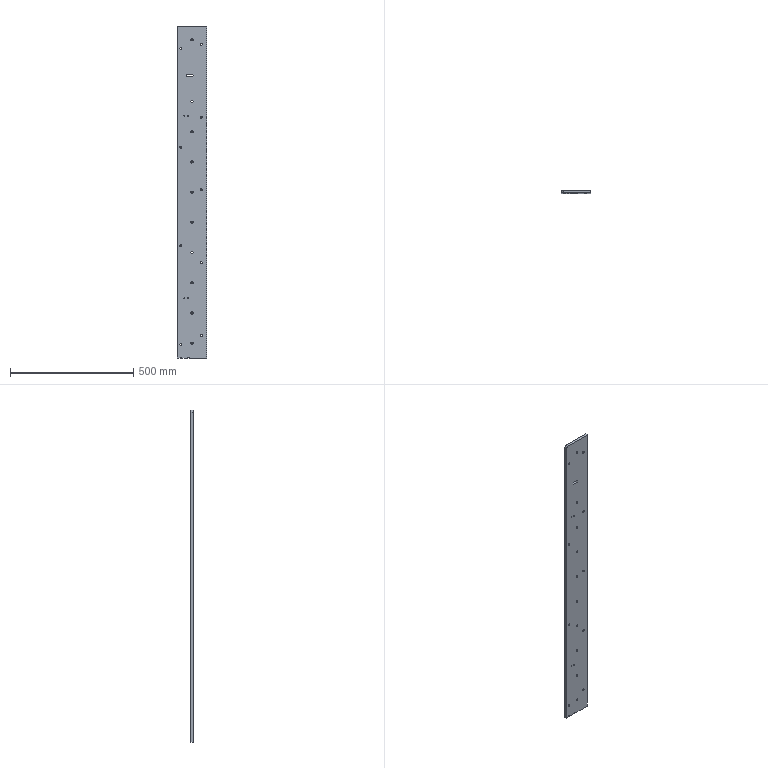Part | STEP file | 1 solid | 66 faces | box 120 x 10 x 1346 mm | volume 1599795 mm3 | cylinder 53 | plane 13 | commonest cylinder face diameters 9 x20 8.4 x10 4.2 x8 8.5 x8 7 x4 2 x2